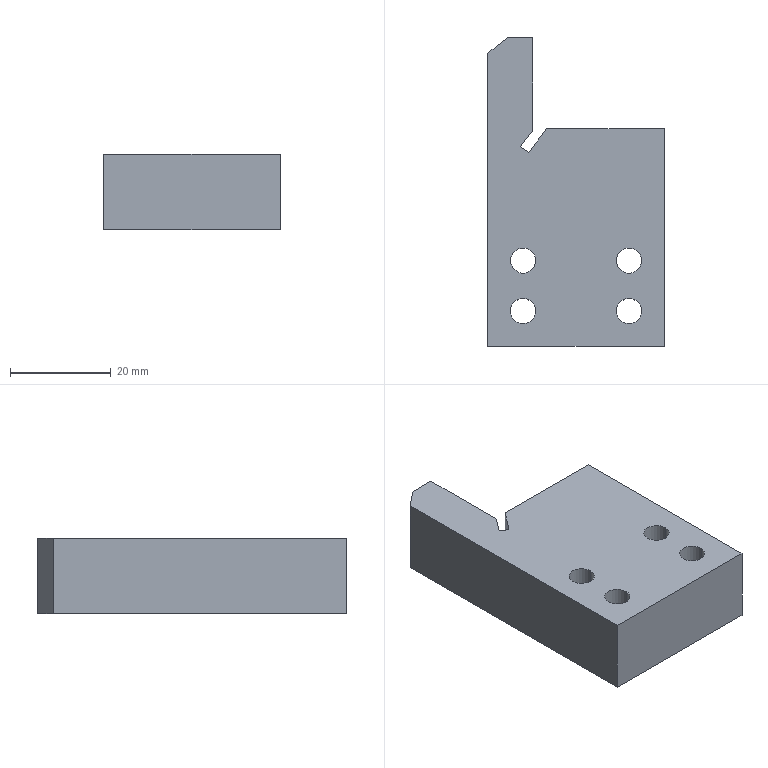Part | SolidWorks | features BaseBody 1 | 1 solid | 20 faces | box 35 x 61.218 x 15 mm | volume 23648 mm3 | plane 12 | cylinder 8 | commonest cylinder face diameters 5 x8
STEP:
#1=CARTESIAN_POINT('',(4.5,7.,15.));
#2=VERTEX_POINT('',#1);
#3=CARTESIAN_POINT('',(9.5,7.,15.));
#4=VERTEX_POINT('',#3);
#5=CARTESIAN_POINT('',(7.,7.,15.));
#6=DIRECTION('',(0.,0.,1.));
#7=DIRECTION('',(-1.,0.,0.));
#8=AXIS2_PLACEMENT_3D('',#5,#6,#7);
#9=CIRCLE('',#8,2.5);
#10=EDGE_CURVE('',#2,#4,#9,.T.);
#11=ORIENTED_EDGE('',*,*,#10,.T.);
#12=CARTESIAN_POINT('',(9.5,7.,0.));
#13=VERTEX_POINT('',#12);
#14=CARTESIAN_POINT('',(9.5,7.,15.));
#15=DIRECTION('',(0.,0.,-1.));
#16=VECTOR('',#15,1000.);
#17=LINE('',#14,#16);
#18=EDGE_CURVE('',#4,#13,#17,.T.);
#19=ORIENTED_EDGE('',*,*,#18,.T.);
#20=CARTESIAN_POINT('',(4.5,7.,0.));
#21=VERTEX_POINT('',#20);
#22=CARTESIAN_POINT('',(7.,7.,0.));
#23=DIRECTION('',(0.,0.,1.));
#24=DIRECTION('',(-1.,0.,0.));
#25=AXIS2_PLACEMENT_3D('',#22,#23,#24);
#26=CIRCLE('',#25,2.5);
#27=EDGE_CURVE('',#21,#13,#26,.T.);
#28=ORIENTED_EDGE('',*,*,#27,.F.);
#29=CARTESIAN_POINT('',(4.5,7.,15.));
#30=DIRECTION('',(0.,0.,-1.));
#31=VECTOR('',#30,1000.);
#32=LINE('',#29,#31);
#33=EDGE_CURVE('',#2,#21,#32,.T.);
#34=ORIENTED_EDGE('',*,*,#33,.F.);
#35=EDGE_LOOP('',(#11,#19,#28,#34));
#36=FACE_OUTER_BOUND('',#35,.T.);
#37=CARTESIAN_POINT('',(7.,7.,15.));
#38=DIRECTION('',(0.,0.,-1.));
#39=DIRECTION('',(-1.,0.,0.));
#40=AXIS2_PLACEMENT_3D('',#37,#38,#39);
#41=CYLINDRICAL_SURFACE('',#40,2.5);
#42=ADVANCED_FACE('',(#36),#41,.F.);
#43=CARTESIAN_POINT('',(25.5,7.,15.));
#44=VERTEX_POINT('',#43);
#45=CARTESIAN_POINT('',(30.5,7.,15.));
#46=VERTEX_POINT('',#45);
#47=CARTESIAN_POINT('',(28.,7.,15.));
#48=DIRECTION('',(0.,0.,1.));
#49=DIRECTION('',(-1.,0.,0.));
#50=AXIS2_PLACEMENT_3D('',#47,#48,#49);
#51=CIRCLE('',#50,2.5);
#52=EDGE_CURVE('',#44,#46,#51,.T.);
#53=ORIENTED_EDGE('',*,*,#52,.T.);
#54=CARTESIAN_POINT('',(30.5,7.,0.));
#55=VERTEX_POINT('',#54);
#56=CARTESIAN_POINT('',(30.5,7.,15.));
#57=DIRECTION('',(0.,0.,-1.));
#58=VECTOR('',#57,1000.);
#59=LINE('',#56,#58);
#60=EDGE_CURVE('',#46,#55,#59,.T.);
#61=ORIENTED_EDGE('',*,*,#60,.T.);
#62=CARTESIAN_POINT('',(25.5,7.,0.));
#63=VERTEX_POINT('',#62);
#64=CARTESIAN_POINT('',(28.,7.,0.));
#65=DIRECTION('',(0.,0.,1.));
#66=DIRECTION('',(-1.,0.,0.));
#67=AXIS2_PLACEMENT_3D('',#64,#65,#66);
#68=CIRCLE('',#67,2.5);
#69=EDGE_CURVE('',#63,#55,#68,.T.);
#70=ORIENTED_EDGE('',*,*,#69,.F.);
#71=CARTESIAN_POINT('',(25.5,7.,15.));
#72=DIRECTION('',(0.,0.,-1.));
#73=VECTOR('',#72,1000.);
#74=LINE('',#71,#73);
#75=EDGE_CURVE('',#44,#63,#74,.T.);
#76=ORIENTED_EDGE('',*,*,#75,.F.);
#77=EDGE_LOOP('',(#53,#61,#70,#76));
#78=FACE_OUTER_BOUND('',#77,.T.);
#79=CARTESIAN_POINT('',(28.,7.,15.));
#80=DIRECTION('',(0.,0.,-1.));
#81=DIRECTION('',(-1.,0.,0.));
#82=AXIS2_PLACEMENT_3D('',#79,#80,#81);
#83=CYLINDRICAL_SURFACE('',#82,2.5);
#84=ADVANCED_FACE('',(#78),#83,.F.);
#85=CARTESIAN_POINT('',(4.52,17.,15.));
#86=VERTEX_POINT('',#85);
#87=CARTESIAN_POINT('',(9.52,17.,15.));
#88=VERTEX_POINT('',#87);
#89=CARTESIAN_POINT('',(7.02,17.,15.));
#90=DIRECTION('',(0.,0.,1.));
#91=DIRECTION('',(-1.,0.,0.));
#92=AXIS2_PLACEMENT_3D('',#89,#90,#91);
#93=CIRCLE('',#92,2.5);
#94=EDGE_CURVE('',#86,#88,#93,.T.);
#95=ORIENTED_EDGE('',*,*,#94,.T.);
#96=CARTESIAN_POINT('',(9.52,17.,0.));
#97=VERTEX_POINT('',#96);
#98=CARTESIAN_POINT('',(9.52,17.,15.));
#99=DIRECTION('',(0.,0.,-1.));
#100=VECTOR('',#99,1000.);
#101=LINE('',#98,#100);
#102=EDGE_CURVE('',#88,#97,#101,.T.);
#103=ORIENTED_EDGE('',*,*,#102,.T.);
#104=CARTESIAN_POINT('',(4.52,17.,0.));
#105=VERTEX_POINT('',#104);
#106=CARTESIAN_POINT('',(7.02,17.,0.));
#107=DIRECTION('',(0.,0.,1.));
#108=DIRECTION('',(-1.,0.,0.));
#109=AXIS2_PLACEMENT_3D('',#106,#107,#108);
#110=CIRCLE('',#109,2.5);
#111=EDGE_CURVE('',#105,#97,#110,.T.);
#112=ORIENTED_EDGE('',*,*,#111,.F.);
#113=CARTESIAN_POINT('',(4.52,17.,15.));
#114=DIRECTION('',(0.,0.,-1.));
#115=VECTOR('',#114,1000.);
#116=LINE('',#113,#115);
#117=EDGE_CURVE('',#86,#105,#116,.T.);
#118=ORIENTED_EDGE('',*,*,#117,.F.);
#119=EDGE_LOOP('',(#95,#103,#112,#118));
#120=FACE_OUTER_BOUND('',#119,.T.);
#121=CARTESIAN_POINT('',(7.02,17.,15.));
#122=DIRECTION('',(0.,0.,-1.));
#123=DIRECTION('',(-1.,0.,0.));
#124=AXIS2_PLACEMENT_3D('',#121,#122,#123);
#125=CYLINDRICAL_SURFACE('',#124,2.5);
#126=ADVANCED_FACE('',(#120),#125,.F.);
#127=CARTESIAN_POINT('',(25.5,17.,15.));
#128=VERTEX_POINT('',#127);
#129=CARTESIAN_POINT('',(30.5,17.,15.));
#130=VERTEX_POINT('',#129);
#131=CARTESIAN_POINT('',(28.,17.,15.));
#132=DIRECTION('',(0.,0.,1.));
#133=DIRECTION('',(-1.,0.,0.));
#134=AXIS2_PLACEMENT_3D('',#131,#132,#133);
#135=CIRCLE('',#134,2.5);
#136=EDGE_CURVE('',#128,#130,#135,.T.);
#137=ORIENTED_EDGE('',*,*,#136,.T.);
#138=CARTESIAN_POINT('',(30.5,17.,0.));
#139=VERTEX_POINT('',#138);
#140=CARTESIAN_POINT('',(30.5,17.,15.));
#141=DIRECTION('',(0.,0.,-1.));
#142=VECTOR('',#141,1000.);
#143=LINE('',#140,#142);
#144=EDGE_CURVE('',#130,#139,#143,.T.);
#145=ORIENTED_EDGE('',*,*,#144,.T.);
#146=CARTESIAN_POINT('',(25.5,17.,0.));
#147=VERTEX_POINT('',#146);
#148=CARTESIAN_POINT('',(28.,17.,0.));
#149=DIRECTION('',(0.,0.,1.));
#150=DIRECTION('',(-1.,0.,0.));
#151=AXIS2_PLACEMENT_3D('',#148,#149,#150);
#152=CIRCLE('',#151,2.5);
#153=EDGE_CURVE('',#147,#139,#152,.T.);
#154=ORIENTED_EDGE('',*,*,#153,.F.);
#155=CARTESIAN_POINT('',(25.5,17.,15.));
#156=DIRECTION('',(0.,0.,-1.));
#157=VECTOR('',#156,1000.);
#158=LINE('',#155,#157);
#159=EDGE_CURVE('',#128,#147,#158,.T.);
#160=ORIENTED_EDGE('',*,*,#159,.F.);
#161=EDGE_LOOP('',(#137,#145,#154,#160));
#162=FACE_OUTER_BOUND('',#161,.T.);
#163=CARTESIAN_POINT('',(28.,17.,15.));
#164=DIRECTION('',(0.,0.,-1.));
#165=DIRECTION('',(-1.,0.,0.));
#166=AXIS2_PLACEMENT_3D('',#163,#164,#165);
#167=CYLINDRICAL_SURFACE('',#166,2.5);
#168=ADVANCED_FACE('',(#162),#167,.F.);
#169=CARTESIAN_POINT('',(35.,43.14,15.));
#170=VERTEX_POINT('',#169);
#171=CARTESIAN_POINT('',(35.,0.,15.));
#172=VERTEX_POINT('',#171);
#173=CARTESIAN_POINT('',(35.,0.,15.));
#174=DIRECTION('',(0.,-1.,0.));
#175=VECTOR('',#174,1000.);
#176=LINE('',#173,#175);
#177=EDGE_CURVE('',#170,#172,#176,.T.);
#178=ORIENTED_EDGE('',*,*,#177,.F.);
#179=CARTESIAN_POINT('',(11.7,43.14,15.));
#180=VERTEX_POINT('',#179);
#181=CARTESIAN_POINT('',(0.,43.14,15.));
#182=DIRECTION('',(1.,0.,0.));
#183=VECTOR('',#182,1000.);
#184=LINE('',#181,#183);
#185=EDGE_CURVE('',#180,#170,#184,.T.);
#186=ORIENTED_EDGE('',*,*,#185,.F.);
#187=CARTESIAN_POINT('',(8.118,38.486,15.));
#188=VERTEX_POINT('',#187);
#189=CARTESIAN_POINT('',(8.118,38.486,15.));
#190=DIRECTION('',(0.6099,0.7924,0.));
#191=VECTOR('',#190,1000.);
#192=LINE('',#189,#191);
#193=EDGE_CURVE('',#188,#180,#192,.T.);
#194=ORIENTED_EDGE('',*,*,#193,.F.);
#195=CARTESIAN_POINT('',(6.44,39.575,15.));
#196=VERTEX_POINT('',#195);
#197=CARTESIAN_POINT('',(6.44,39.575,15.));
#198=DIRECTION('',(0.839,-0.5441,0.));
#199=VECTOR('',#198,1000.);
#200=LINE('',#197,#199);
#201=EDGE_CURVE('',#196,#188,#200,.T.);
#202=ORIENTED_EDGE('',*,*,#201,.F.);
#203=CARTESIAN_POINT('',(8.94,42.818,15.));
#204=VERTEX_POINT('',#203);
#205=CARTESIAN_POINT('',(8.94,42.818,15.));
#206=DIRECTION('',(-0.6105,-0.7921,0.));
#207=VECTOR('',#206,1000.);
#208=LINE('',#205,#207);
#209=EDGE_CURVE('',#204,#196,#208,.T.);
#210=ORIENTED_EDGE('',*,*,#209,.F.);
#211=CARTESIAN_POINT('',(8.94,61.218,15.));
#212=VERTEX_POINT('',#211);
#213=CARTESIAN_POINT('',(8.94,0.,15.));
#214=DIRECTION('',(0.,-1.,0.));
#215=VECTOR('',#214,1000.);
#216=LINE('',#213,#215);
#217=EDGE_CURVE('',#212,#204,#216,.T.);
#218=ORIENTED_EDGE('',*,*,#217,.F.);
#219=CARTESIAN_POINT('',(3.94,61.218,15.));
#220=VERTEX_POINT('',#219);
#221=CARTESIAN_POINT('',(0.,61.218,15.));
#222=DIRECTION('',(1.,0.,0.));
#223=VECTOR('',#222,1000.);
#224=LINE('',#221,#223);
#225=EDGE_CURVE('',#220,#212,#224,.T.);
#226=ORIENTED_EDGE('',*,*,#225,.F.);
#227=CARTESIAN_POINT('',(0.,58.14,15.));
#228=VERTEX_POINT('',#227);
#229=CARTESIAN_POINT('',(0.,58.14,15.));
#230=DIRECTION('',(0.788,0.6157,0.));
#231=VECTOR('',#230,1000.);
#232=LINE('',#229,#231);
#233=EDGE_CURVE('',#228,#220,#232,.T.);
#234=ORIENTED_EDGE('',*,*,#233,.F.);
#235=CARTESIAN_POINT('',(0.,0.,15.));
#236=VERTEX_POINT('',#235);
#237=CARTESIAN_POINT('',(0.,0.,15.));
#238=DIRECTION('',(0.,1.,0.));
#239=VECTOR('',#238,1000.);
#240=LINE('',#237,#239);
#241=EDGE_CURVE('',#236,#228,#240,.T.);
#242=ORIENTED_EDGE('',*,*,#241,.F.);
#243=CARTESIAN_POINT('',(0.,0.,15.));
#244=DIRECTION('',(-1.,0.,0.));
#245=VECTOR('',#244,1000.);
#246=LINE('',#243,#245);
#247=EDGE_CURVE('',#172,#236,#246,.T.);
#248=ORIENTED_EDGE('',*,*,#247,.F.);
#249=EDGE_LOOP('',(#178,#186,#194,#202,#210,#218,#226,#234,#242,#248));
#250=FACE_OUTER_BOUND('',#249,.T.);
#251=ORIENTED_EDGE('',*,*,#10,.F.);
#252=CARTESIAN_POINT('',(7.,7.,15.));
#253=DIRECTION('',(0.,0.,1.));
#254=DIRECTION('',(-1.,0.,0.));
#255=AXIS2_PLACEMENT_3D('',#252,#253,#254);
#256=CIRCLE('',#255,2.5);
#257=EDGE_CURVE('',#4,#2,#256,.T.);
#258=ORIENTED_EDGE('',*,*,#257,.F.);
#259=EDGE_LOOP('',(#251,#258));
#260=FACE_BOUND('',#259,.T.);
#261=ORIENTED_EDGE('',*,*,#52,.F.);
#262=CARTESIAN_POINT('',(28.,7.,15.));
#263=DIRECTION('',(0.,0.,1.));
#264=DIRECTION('',(-1.,0.,0.));
#265=AXIS2_PLACEMENT_3D('',#262,#263,#264);
#266=CIRCLE('',#265,2.5);
#267=EDGE_CURVE('',#46,#44,#266,.T.);
#268=ORIENTED_EDGE('',*,*,#267,.F.);
#269=EDGE_LOOP('',(#261,#268));
#270=FACE_BOUND('',#269,.T.);
#271=ORIENTED_EDGE('',*,*,#94,.F.);
#272=CARTESIAN_POINT('',(7.02,17.,15.));
#273=DIRECTION('',(0.,0.,1.));
#274=DIRECTION('',(-1.,0.,0.));
#275=AXIS2_PLACEMENT_3D('',#272,#273,#274);
#276=CIRCLE('',#275,2.5);
#277=EDGE_CURVE('',#88,#86,#276,.T.);
#278=ORIENTED_EDGE('',*,*,#277,.F.);
#279=EDGE_LOOP('',(#271,#278));
#280=FACE_BOUND('',#279,.T.);
#281=ORIENTED_EDGE('',*,*,#136,.F.);
#282=CARTESIAN_POINT('',(28.,17.,15.));
#283=DIRECTION('',(0.,0.,1.));
#284=DIRECTION('',(-1.,0.,0.));
#285=AXIS2_PLACEMENT_3D('',#282,#283,#284);
#286=CIRCLE('',#285,2.5);
#287=EDGE_CURVE('',#130,#128,#286,.T.);
#288=ORIENTED_EDGE('',*,*,#287,.F.);
#289=EDGE_LOOP('',(#281,#288));
#290=FACE_BOUND('',#289,.T.);
#291=CARTESIAN_POINT('',(0.,0.,15.));
#292=DIRECTION('',(0.,0.,-1.));
#293=DIRECTION('',(-1.,0.,0.));
#294=AXIS2_PLACEMENT_3D('',#291,#292,#293);
#295=PLANE('',#294);
#296=ADVANCED_FACE('',(#250,#260,#270,#280,#290),#295,.F.);
#297=ORIENTED_EDGE('',*,*,#247,.T.);
#298=CARTESIAN_POINT('',(0.,0.,0.));
#299=VERTEX_POINT('',#298);
#300=CARTESIAN_POINT('',(0.,0.,15.));
#301=DIRECTION('',(0.,0.,-1.));
#302=VECTOR('',#301,1000.);
#303=LINE('',#300,#302);
#304=EDGE_CURVE('',#236,#299,#303,.T.);
#305=ORIENTED_EDGE('',*,*,#304,.T.);
#306=CARTESIAN_POINT('',(35.,0.,0.));
#307=VERTEX_POINT('',#306);
#308=CARTESIAN_POINT('',(35.,0.,0.));
#309=DIRECTION('',(1.,0.,0.));
#310=VECTOR('',#309,1000.);
#311=LINE('',#308,#310);
#312=EDGE_CURVE('',#299,#307,#311,.T.);
#313=ORIENTED_EDGE('',*,*,#312,.T.);
#314=CARTESIAN_POINT('',(35.,0.,15.));
#315=DIRECTION('',(0.,0.,1.));
#316=VECTOR('',#315,1000.);
#317=LINE('',#314,#316);
#318=EDGE_CURVE('',#307,#172,#317,.T.);
#319=ORIENTED_EDGE('',*,*,#318,.T.);
#320=EDGE_LOOP('',(#297,#305,#313,#319));
#321=FACE_OUTER_BOUND('',#320,.T.);
#322=CARTESIAN_POINT('',(35.,0.,15.));
#323=DIRECTION('',(0.,-1.,0.));
#324=DIRECTION('',(0.,0.,-1.));
#325=AXIS2_PLACEMENT_3D('',#322,#323,#324);
#326=PLANE('',#325);
#327=ADVANCED_FACE('',(#321),#326,.T.);
#328=ORIENTED_EDGE('',*,*,#177,.T.);
#329=ORIENTED_EDGE('',*,*,#318,.F.);
#330=CARTESIAN_POINT('',(35.,43.14,0.));
#331=VERTEX_POINT('',#330);
#332=CARTESIAN_POINT('',(35.,43.14,0.));
#333=DIRECTION('',(0.,1.,0.));
#334=VECTOR('',#333,1000.);
#335=LINE('',#332,#334);
#336=EDGE_CURVE('',#307,#331,#335,.T.);
#337=ORIENTED_EDGE('',*,*,#336,.T.);
#338=CARTESIAN_POINT('',(35.,43.14,15.));
#339=DIRECTION('',(0.,0.,1.));
#340=VECTOR('',#339,1000.);
#341=LINE('',#338,#340);
#342=EDGE_CURVE('',#331,#170,#341,.T.);
#343=ORIENTED_EDGE('',*,*,#342,.T.);
#344=EDGE_LOOP('',(#328,#329,#337,#343));
#345=FACE_OUTER_BOUND('',#344,.T.);
#346=CARTESIAN_POINT('',(35.,43.14,15.));
#347=DIRECTION('',(1.,0.,0.));
#348=DIRECTION('',(0.,0.,-1.));
#349=AXIS2_PLACEMENT_3D('',#346,#347,#348);
#350=PLANE('',#349);
#351=ADVANCED_FACE('',(#345),#350,.T.);
#352=ORIENTED_EDGE('',*,*,#185,.T.);
#353=ORIENTED_EDGE('',*,*,#342,.F.);
#354=CARTESIAN_POINT('',(11.7,43.14,0.));
#355=VERTEX_POINT('',#354);
#356=CARTESIAN_POINT('',(11.7,43.14,0.));
#357=DIRECTION('',(-1.,0.,0.));
#358=VECTOR('',#357,1000.);
#359=LINE('',#356,#358);
#360=EDGE_CURVE('',#331,#355,#359,.T.);
#361=ORIENTED_EDGE('',*,*,#360,.T.);
#362=CARTESIAN_POINT('',(11.7,43.14,15.));
#363=DIRECTION('',(0.,0.,1.));
#364=VECTOR('',#363,1000.);
#365=LINE('',#362,#364);
#366=EDGE_CURVE('',#355,#180,#365,.T.);
#367=ORIENTED_EDGE('',*,*,#366,.T.);
#368=EDGE_LOOP('',(#352,#353,#361,#367));
#369=FACE_OUTER_BOUND('',#368,.T.);
#370=CARTESIAN_POINT('',(11.7,43.14,15.));
#371=DIRECTION('',(0.,1.,0.));
#372=DIRECTION('',(-1.,0.,0.));
#373=AXIS2_PLACEMENT_3D('',#370,#371,#372);
#374=PLANE('',#373);
#375=ADVANCED_FACE('',(#369),#374,.T.);
#376=ORIENTED_EDGE('',*,*,#193,.T.);
#377=ORIENTED_EDGE('',*,*,#366,.F.);
#378=CARTESIAN_POINT('',(8.118,38.486,0.));
#379=VERTEX_POINT('',#378);
#380=CARTESIAN_POINT('',(8.118,38.486,0.));
#381=DIRECTION('',(-0.6099,-0.7924,0.));
#382=VECTOR('',#381,1000.);
#383=LINE('',#380,#382);
#384=EDGE_CURVE('',#355,#379,#383,.T.);
#385=ORIENTED_EDGE('',*,*,#384,.T.);
#386=CARTESIAN_POINT('',(8.118,38.486,15.));
#387=DIRECTION('',(0.,0.,1.));
#388=VECTOR('',#387,1000.);
#389=LINE('',#386,#388);
#390=EDGE_CURVE('',#379,#188,#389,.T.);
#391=ORIENTED_EDGE('',*,*,#390,.T.);
#392=EDGE_LOOP('',(#376,#377,#385,#391));
#393=FACE_OUTER_BOUND('',#392,.T.);
#394=CARTESIAN_POINT('',(8.118,38.486,15.));
#395=DIRECTION('',(-0.7924,0.6099,0.));
#396=DIRECTION('',(-0.6099,-0.7924,0.));
#397=AXIS2_PLACEMENT_3D('',#394,#395,#396);
#398=PLANE('',#397);
#399=ADVANCED_FACE('',(#393),#398,.T.);
#400=ORIENTED_EDGE('',*,*,#201,.T.);
#401=ORIENTED_EDGE('',*,*,#390,.F.);
#402=CARTESIAN_POINT('',(6.44,39.575,0.));
#403=VERTEX_POINT('',#402);
#404=CARTESIAN_POINT('',(6.44,39.575,0.));
#405=DIRECTION('',(-0.839,0.5441,0.));
#406=VECTOR('',#405,1000.);
#407=LINE('',#404,#406);
#408=EDGE_CURVE('',#379,#403,#407,.T.);
#409=ORIENTED_EDGE('',*,*,#408,.T.);
#410=CARTESIAN_POINT('',(6.44,39.575,15.));
#411=DIRECTION('',(0.,0.,1.));
#412=VECTOR('',#411,1000.);
#413=LINE('',#410,#412);
#414=EDGE_CURVE('',#403,#196,#413,.T.);
#415=ORIENTED_EDGE('',*,*,#414,.T.);
#416=EDGE_LOOP('',(#400,#401,#409,#415));
#417=FACE_OUTER_BOUND('',#416,.T.);
#418=CARTESIAN_POINT('',(6.44,39.575,15.));
#419=DIRECTION('',(0.5441,0.839,0.));
#420=DIRECTION('',(-0.839,0.5441,0.));
#421=AXIS2_PLACEMENT_3D('',#418,#419,#420);
#422=PLANE('',#421);
#423=ADVANCED_FACE('',(#417),#422,.T.);
#424=ORIENTED_EDGE('',*,*,#209,.T.);
#425=ORIENTED_EDGE('',*,*,#414,.F.);
#426=CARTESIAN_POINT('',(8.94,42.818,0.));
#427=VERTEX_POINT('',#426);
#428=CARTESIAN_POINT('',(8.94,42.818,0.));
#429=DIRECTION('',(0.6105,0.7921,0.));
#430=VECTOR('',#429,1000.);
#431=LINE('',#428,#430);
#432=EDGE_CURVE('',#403,#427,#431,.T.);
#433=ORIENTED_EDGE('',*,*,#432,.T.);
#434=CARTESIAN_POINT('',(8.94,42.818,15.));
#435=DIRECTION('',(0.,0.,1.));
#436=VECTOR('',#435,1000.);
#437=LINE('',#434,#436);
#438=EDGE_CURVE('',#427,#204,#437,.T.);
#439=ORIENTED_EDGE('',*,*,#438,.T.);
#440=EDGE_LOOP('',(#424,#425,#433,#439));
#441=FACE_OUTER_BOUND('',#440,.T.);
#442=CARTESIAN_POINT('',(8.94,42.818,15.));
#443=DIRECTION('',(0.7921,-0.6105,0.));
#444=DIRECTION('',(0.6105,0.7921,0.));
#445=AXIS2_PLACEMENT_3D('',#442,#443,#444);
#446=PLANE('',#445);
#447=ADVANCED_FACE('',(#441),#446,.T.);
#448=ORIENTED_EDGE('',*,*,#217,.T.);
#449=ORIENTED_EDGE('',*,*,#438,.F.);
#450=CARTESIAN_POINT('',(8.94,61.218,0.));
#451=VERTEX_POINT('',#450);
#452=CARTESIAN_POINT('',(8.94,61.218,0.));
#453=DIRECTION('',(0.,1.,0.));
#454=VECTOR('',#453,1000.);
#455=LINE('',#452,#454);
#456=EDGE_CURVE('',#427,#451,#455,.T.);
#457=ORIENTED_EDGE('',*,*,#456,.T.);
#458=CARTESIAN_POINT('',(8.94,61.218,15.));
#459=DIRECTION('',(0.,0.,1.));
#460=VECTOR('',#459,1000.);
#461=LINE('',#458,#460);
#462=EDGE_CURVE('',#451,#212,#461,.T.);
#463=ORIENTED_EDGE('',*,*,#462,.T.);
#464=EDGE_LOOP('',(#448,#449,#457,#463));
#465=FACE_OUTER_BOUND('',#464,.T.);
#466=CARTESIAN_POINT('',(8.94,61.218,15.));
#467=DIRECTION('',(1.,0.,0.));
#468=DIRECTION('',(0.,1.,0.));
#469=AXIS2_PLACEMENT_3D('',#466,#467,#468);
#470=PLANE('',#469);
#471=ADVANCED_FACE('',(#465),#470,.T.);
#472=ORIENTED_EDGE('',*,*,#225,.T.);
#473=ORIENTED_EDGE('',*,*,#462,.F.);
#474=CARTESIAN_POINT('',(3.94,61.218,0.));
#475=VERTEX_POINT('',#474);
#476=CARTESIAN_POINT('',(3.94,61.218,0.));
#477=DIRECTION('',(-1.,0.,0.));
#478=VECTOR('',#477,1000.);
#479=LINE('',#476,#478);
#480=EDGE_CURVE('',#451,#475,#479,.T.);
#481=ORIENTED_EDGE('',*,*,#480,.T.);
#482=CARTESIAN_POINT('',(3.94,61.218,15.));
#483=DIRECTION('',(0.,0.,1.));
#484=VECTOR('',#483,1000.);
#485=LINE('',#482,#484);
#486=EDGE_CURVE('',#475,#220,#485,.T.);
#487=ORIENTED_EDGE('',*,*,#486,.T.);
#488=EDGE_LOOP('',(#472,#473,#481,#487));
#489=FACE_OUTER_BOUND('',#488,.T.);
#490=CARTESIAN_POINT('',(3.94,61.218,15.));
#491=DIRECTION('',(0.,1.,0.));
#492=DIRECTION('',(0.,0.,1.));
#493=AXIS2_PLACEMENT_3D('',#490,#491,#492);
#494=PLANE('',#493);
#495=ADVANCED_FACE('',(#489),#494,.T.);
#496=ORIENTED_EDGE('',*,*,#233,.T.);
#497=ORIENTED_EDGE('',*,*,#486,.F.);
#498=CARTESIAN_POINT('',(0.,58.14,0.));
#499=VERTEX_POINT('',#498);
#500=CARTESIAN_POINT('',(0.,58.14,0.));
#501=DIRECTION('',(-0.788,-0.6157,0.));
#502=VECTOR('',#501,1000.);
#503=LINE('',#500,#502);
#504=EDGE_CURVE('',#475,#499,#503,.T.);
#505=ORIENTED_EDGE('',*,*,#504,.T.);
#506=CARTESIAN_POINT('',(0.,58.14,15.));
#507=DIRECTION('',(0.,0.,1.));
#508=VECTOR('',#507,1000.);
#509=LINE('',#506,#508);
#510=EDGE_CURVE('',#499,#228,#509,.T.);
#511=ORIENTED_EDGE('',*,*,#510,.T.);
#512=EDGE_LOOP('',(#496,#497,#505,#511));
#513=FACE_OUTER_BOUND('',#512,.T.);
#514=CARTESIAN_POINT('',(0.,58.14,15.));
#515=DIRECTION('',(-0.6157,0.788,0.));
#516=DIRECTION('',(-0.788,-0.6157,0.));
#517=AXIS2_PLACEMENT_3D('',#514,#515,#516);
#518=PLANE('',#517);
#519=ADVANCED_FACE('',(#513),#518,.T.);
#520=ORIENTED_EDGE('',*,*,#241,.T.);
#521=ORIENTED_EDGE('',*,*,#510,.F.);
#522=CARTESIAN_POINT('',(0.,0.,0.));
#523=DIRECTION('',(0.,-1.,0.));
#524=VECTOR('',#523,1000.);
#525=LINE('',#522,#524);
#526=EDGE_CURVE('',#499,#299,#525,.T.);
#527=ORIENTED_EDGE('',*,*,#526,.T.);
#528=ORIENTED_EDGE('',*,*,#304,.F.);
#529=EDGE_LOOP('',(#520,#521,#527,#528));
#530=FACE_OUTER_BOUND('',#529,.T.);
#531=CARTESIAN_POINT('',(0.,0.,15.));
#532=DIRECTION('',(-1.,0.,0.));
#533=DIRECTION('',(0.,0.,1.));
#534=AXIS2_PLACEMENT_3D('',#531,#532,#533);
#535=PLANE('',#534);
#536=ADVANCED_FACE('',(#530),#535,.T.);
#537=ORIENTED_EDGE('',*,*,#18,.F.);
#538=ORIENTED_EDGE('',*,*,#257,.T.);
#539=ORIENTED_EDGE('',*,*,#33,.T.);
#540=CARTESIAN_POINT('',(7.,7.,0.));
#541=DIRECTION('',(0.,0.,1.));
#542=DIRECTION('',(-1.,0.,0.));
#543=AXIS2_PLACEMENT_3D('',#540,#541,#542);
#544=CIRCLE('',#543,2.5);
#545=EDGE_CURVE('',#13,#21,#544,.T.);
#546=ORIENTED_EDGE('',*,*,#545,.F.);
#547=EDGE_LOOP('',(#537,#538,#539,#546));
#548=FACE_OUTER_BOUND('',#547,.T.);
#549=CARTESIAN_POINT('',(7.,7.,15.));
#550=DIRECTION('',(0.,0.,-1.));
#551=DIRECTION('',(-1.,0.,0.));
#552=AXIS2_PLACEMENT_3D('',#549,#550,#551);
#553=CYLINDRICAL_SURFACE('',#552,2.5);
#554=ADVANCED_FACE('',(#548),#553,.F.);
#555=ORIENTED_EDGE('',*,*,#60,.F.);
#556=ORIENTED_EDGE('',*,*,#267,.T.);
#557=ORIENTED_EDGE('',*,*,#75,.T.);
#558=CARTESIAN_POINT('',(28.,7.,0.));
#559=DIRECTION('',(0.,0.,1.));
#560=DIRECTION('',(-1.,0.,0.));
#561=AXIS2_PLACEMENT_3D('',#558,#559,#560);
#562=CIRCLE('',#561,2.5);
#563=EDGE_CURVE('',#55,#63,#562,.T.);
#564=ORIENTED_EDGE('',*,*,#563,.F.);
#565=EDGE_LOOP('',(#555,#556,#557,#564));
#566=FACE_OUTER_BOUND('',#565,.T.);
#567=CARTESIAN_POINT('',(28.,7.,15.));
#568=DIRECTION('',(0.,0.,-1.));
#569=DIRECTION('',(-1.,0.,0.));
#570=AXIS2_PLACEMENT_3D('',#567,#568,#569);
#571=CYLINDRICAL_SURFACE('',#570,2.5);
#572=ADVANCED_FACE('',(#566),#571,.F.);
#573=ORIENTED_EDGE('',*,*,#102,.F.);
#574=ORIENTED_EDGE('',*,*,#277,.T.);
#575=ORIENTED_EDGE('',*,*,#117,.T.);
#576=CARTESIAN_POINT('',(7.02,17.,0.));
#577=DIRECTION('',(0.,0.,1.));
#578=DIRECTION('',(-1.,0.,0.));
#579=AXIS2_PLACEMENT_3D('',#576,#577,#578);
#580=CIRCLE('',#579,2.5);
#581=EDGE_CURVE('',#97,#105,#580,.T.);
#582=ORIENTED_EDGE('',*,*,#581,.F.);
#583=EDGE_LOOP('',(#573,#574,#575,#582));
#584=FACE_OUTER_BOUND('',#583,.T.);
#585=CARTESIAN_POINT('',(7.02,17.,15.));
#586=DIRECTION('',(0.,0.,-1.));
#587=DIRECTION('',(-1.,0.,0.));
#588=AXIS2_PLACEMENT_3D('',#585,#586,#587);
#589=CYLINDRICAL_SURFACE('',#588,2.5);
#590=ADVANCED_FACE('',(#584),#589,.F.);
#591=ORIENTED_EDGE('',*,*,#144,.F.);
#592=ORIENTED_EDGE('',*,*,#287,.T.);
#593=ORIENTED_EDGE('',*,*,#159,.T.);
#594=CARTESIAN_POINT('',(28.,17.,0.));
#595=DIRECTION('',(0.,0.,1.));
#596=DIRECTION('',(-1.,0.,0.));
#597=AXIS2_PLACEMENT_3D('',#594,#595,#596);
#598=CIRCLE('',#597,2.5);
#599=EDGE_CURVE('',#139,#147,#598,.T.);
#600=ORIENTED_EDGE('',*,*,#599,.F.);
#601=EDGE_LOOP('',(#591,#592,#593,#600));
#602=FACE_OUTER_BOUND('',#601,.T.);
#603=CARTESIAN_POINT('',(28.,17.,15.));
#604=DIRECTION('',(0.,0.,-1.));
#605=DIRECTION('',(-1.,0.,0.));
#606=AXIS2_PLACEMENT_3D('',#603,#604,#605);
#607=CYLINDRICAL_SURFACE('',#606,2.5);
#608=ADVANCED_FACE('',(#602),#607,.F.);
#609=ORIENTED_EDGE('',*,*,#360,.F.);
#610=ORIENTED_EDGE('',*,*,#336,.F.);
#611=ORIENTED_EDGE('',*,*,#312,.F.);
#612=ORIENTED_EDGE('',*,*,#526,.F.);
#613=ORIENTED_EDGE('',*,*,#504,.F.);
#614=ORIENTED_EDGE('',*,*,#480,.F.);
#615=ORIENTED_EDGE('',*,*,#456,.F.);
#616=ORIENTED_EDGE('',*,*,#432,.F.);
#617=ORIENTED_EDGE('',*,*,#408,.F.);
#618=ORIENTED_EDGE('',*,*,#384,.F.);
#619=EDGE_LOOP('',(#609,#610,#611,#612,#613,#614,#615,#616,#617,#618));
#620=FACE_OUTER_BOUND('',#619,.T.);
#621=ORIENTED_EDGE('',*,*,#27,.T.);
#622=ORIENTED_EDGE('',*,*,#545,.T.);
#623=EDGE_LOOP('',(#621,#622));
#624=FACE_BOUND('',#623,.T.);
#625=ORIENTED_EDGE('',*,*,#69,.T.);
#626=ORIENTED_EDGE('',*,*,#563,.T.);
#627=EDGE_LOOP('',(#625,#626));
#628=FACE_BOUND('',#627,.T.);
#629=ORIENTED_EDGE('',*,*,#111,.T.);
#630=ORIENTED_EDGE('',*,*,#581,.T.);
#631=EDGE_LOOP('',(#629,#630));
#632=FACE_BOUND('',#631,.T.);
#633=ORIENTED_EDGE('',*,*,#153,.T.);
#634=ORIENTED_EDGE('',*,*,#599,.T.);
#635=EDGE_LOOP('',(#633,#634));
#636=FACE_BOUND('',#635,.T.);
#637=CARTESIAN_POINT('',(0.,0.,0.));
#638=DIRECTION('',(0.,0.,-1.));
#639=DIRECTION('',(-1.,0.,0.));
#640=AXIS2_PLACEMENT_3D('',#637,#638,#639);
#641=PLANE('',#640);
#642=ADVANCED_FACE('',(#620,#624,#628,#632,#636),#641,.T.);
#643=CLOSED_SHELL('',(#42,#84,#126,#168,#296,#327,#351,#375,#399,#423,#447,#471,#495,#519,#536,#554,#572,#590,#608,#642));
#644=MANIFOLD_SOLID_BREP('',#643);
#645=CARTESIAN_POINT('',(0.,0.,0.));
#646=DIRECTION('',(0.,0.,1.));
#647=DIRECTION('',(1.,0.,0.));
#648=AXIS2_PLACEMENT_3D('',#645,#646,#647);
#649=(LENGTH_UNIT()NAMED_UNIT(*)SI_UNIT(.MILLI.,.METRE.));
#650=UNCERTAINTY_MEASURE_WITH_UNIT(LENGTH_MEASURE(0.00001),#649,'','');
#651=(NAMED_UNIT(*)PLANE_ANGLE_UNIT()SI_UNIT($,.RADIAN.));
#652=(NAMED_UNIT(*)SI_UNIT($,.STERADIAN.)SOLID_ANGLE_UNIT());
#653=(GEOMETRIC_REPRESENTATION_CONTEXT(3)GLOBAL_UNCERTAINTY_ASSIGNED_CONTEXT((#650))GLOBAL_UNIT_ASSIGNED_CONTEXT((#649,#651,#652))REPRESENTATION_CONTEXT('',''));
#654=ADVANCED_BREP_SHAPE_REPRESENTATION('',(#644,#648),#653);